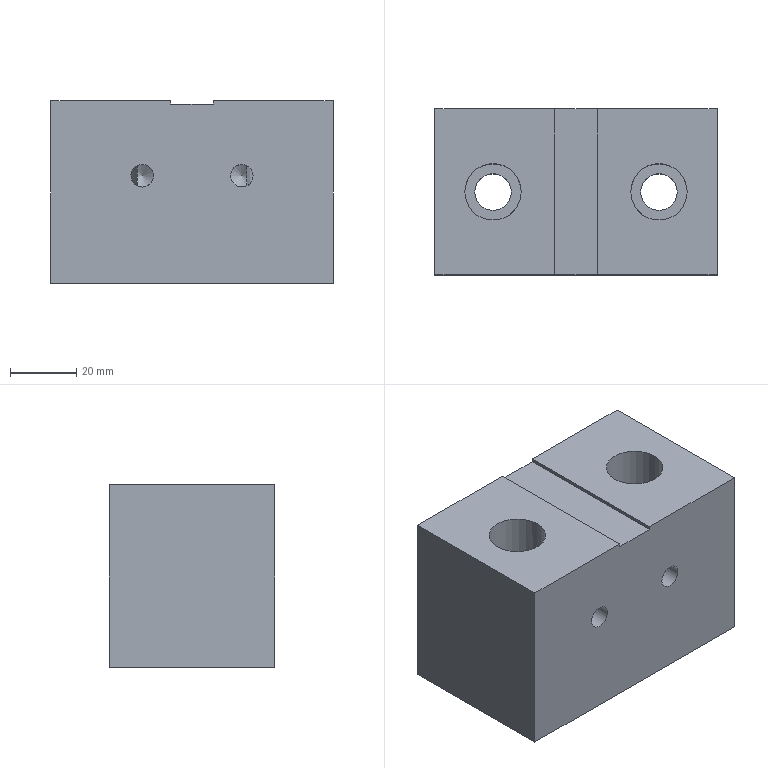Part | STEP file | 1 solid | 20 faces | box 85 x 50 x 55 mm | volume 210302 mm3 | plane 12 | cylinder 6 | cone 2 | commonest cylinder face diameters 6.8 x2 11 x2 17 x2
STEP:
#1=CARTESIAN_POINT('',(-370.,-292.5,-47.));
#2=VERTEX_POINT('',#1);
#3=CARTESIAN_POINT('',(-285.,-292.5,-47.));
#4=VERTEX_POINT('',#3);
#5=CARTESIAN_POINT('',(-383.,-292.5,-47.));
#6=DIRECTION('',(1.,0.,0.));
#7=VECTOR('',#6,1.);
#8=LINE('',#5,#7);
#9=EDGE_CURVE('',#2,#4,#8,.T.);
#10=ORIENTED_EDGE('',*,*,#9,.T.);
#11=CARTESIAN_POINT('',(-285.,-292.5,8.));
#12=VERTEX_POINT('',#11);
#13=CARTESIAN_POINT('',(-285.,-292.5,24.2));
#14=DIRECTION('',(0.,0.,1.));
#15=VECTOR('',#14,1.);
#16=LINE('',#13,#15);
#17=EDGE_CURVE('',#4,#12,#16,.T.);
#18=ORIENTED_EDGE('',*,*,#17,.T.);
#19=CARTESIAN_POINT('',(-321.15,-292.5,8.));
#20=VERTEX_POINT('',#19);
#21=CARTESIAN_POINT('',(-335.,-292.5,8.));
#22=DIRECTION('',(-1.,0.,0.));
#23=VECTOR('',#22,1.);
#24=LINE('',#21,#23);
#25=EDGE_CURVE('',#12,#20,#24,.T.);
#26=ORIENTED_EDGE('',*,*,#25,.T.);
#27=CARTESIAN_POINT('',(-321.15,-292.5,7.));
#28=VERTEX_POINT('',#27);
#29=CARTESIAN_POINT('',(-321.15,-292.5,24.2));
#30=DIRECTION('',(0.,0.,1.));
#31=VECTOR('',#30,1.);
#32=LINE('',#29,#31);
#33=EDGE_CURVE('',#28,#20,#32,.T.);
#34=ORIENTED_EDGE('',*,*,#33,.F.);
#35=CARTESIAN_POINT('',(-333.85,-292.5,7.));
#36=VERTEX_POINT('',#35);
#37=CARTESIAN_POINT('',(-383.,-292.5,7.));
#38=DIRECTION('',(1.,0.,0.));
#39=VECTOR('',#38,1.);
#40=LINE('',#37,#39);
#41=EDGE_CURVE('',#36,#28,#40,.T.);
#42=ORIENTED_EDGE('',*,*,#41,.F.);
#43=CARTESIAN_POINT('',(-333.85,-292.5,8.));
#44=VERTEX_POINT('',#43);
#45=CARTESIAN_POINT('',(-333.85,-292.5,24.2));
#46=DIRECTION('',(0.,0.,1.));
#47=VECTOR('',#46,1.);
#48=LINE('',#45,#47);
#49=EDGE_CURVE('',#36,#44,#48,.T.);
#50=ORIENTED_EDGE('',*,*,#49,.T.);
#51=CARTESIAN_POINT('',(-370.,-292.5,8.));
#52=VERTEX_POINT('',#51);
#53=CARTESIAN_POINT('',(-335.,-292.5,8.));
#54=DIRECTION('',(-1.,0.,0.));
#55=VECTOR('',#54,1.);
#56=LINE('',#53,#55);
#57=EDGE_CURVE('',#44,#52,#56,.T.);
#58=ORIENTED_EDGE('',*,*,#57,.T.);
#59=CARTESIAN_POINT('',(-370.,-292.5,24.2));
#60=DIRECTION('',(0.,0.,1.));
#61=VECTOR('',#60,1.);
#62=LINE('',#59,#61);
#63=EDGE_CURVE('',#2,#52,#62,.T.);
#64=ORIENTED_EDGE('',*,*,#63,.F.);
#65=EDGE_LOOP('',(#10,#18,#26,#34,#42,#50,#58,#64));
#66=FACE_BOUND('',#65,.T.);
#67=CARTESIAN_POINT('',(-339.1,-292.5,-14.6));
#68=VERTEX_POINT('',#67);
#69=CARTESIAN_POINT('',(-342.5,-292.5,-14.6));
#70=DIRECTION('',(0.,1.,0.));
#71=DIRECTION('',(1.,0.,0.));
#72=AXIS2_PLACEMENT_3D('',#69,#70,#71);
#73=CIRCLE('',#72,3.4);
#74=EDGE_CURVE('',#68,#68,#73,.T.);
#75=ORIENTED_EDGE('',*,*,#74,.T.);
#76=EDGE_LOOP('',(#75));
#77=FACE_BOUND('',#76,.T.);
#78=CARTESIAN_POINT('',(-309.1,-292.5,-14.6));
#79=VERTEX_POINT('',#78);
#80=CARTESIAN_POINT('',(-312.5,-292.5,-14.6));
#81=DIRECTION('',(0.,1.,0.));
#82=DIRECTION('',(1.,0.,0.));
#83=AXIS2_PLACEMENT_3D('',#80,#81,#82);
#84=CIRCLE('',#83,3.4);
#85=EDGE_CURVE('',#79,#79,#84,.T.);
#86=ORIENTED_EDGE('',*,*,#85,.T.);
#87=EDGE_LOOP('',(#86));
#88=FACE_BOUND('',#87,.T.);
#89=CARTESIAN_POINT('',(-383.,-292.5,24.2));
#90=DIRECTION('',(0.,-1.,0.));
#91=DIRECTION('',(0.,0.,-1.));
#92=AXIS2_PLACEMENT_3D('',#89,#90,#91);
#93=PLANE('',#92);
#94=ADVANCED_FACE('',(#66,#77,#88),#93,.T.);
#95=CARTESIAN_POINT('',(-361.,-267.5,8.));
#96=VERTEX_POINT('',#95);
#97=CARTESIAN_POINT('',(-352.5,-267.5,8.));
#98=DIRECTION('',(0.,0.,-1.));
#99=DIRECTION('',(-1.,0.,0.));
#100=AXIS2_PLACEMENT_3D('',#97,#98,#99);
#101=CIRCLE('',#100,8.5);
#102=EDGE_CURVE('',#96,#96,#101,.T.);
#103=ORIENTED_EDGE('',*,*,#102,.T.);
#104=EDGE_LOOP('',(#103));
#105=FACE_BOUND('',#104,.T.);
#106=CARTESIAN_POINT('',(-370.,-242.5,8.));
#107=VERTEX_POINT('',#106);
#108=CARTESIAN_POINT('',(-333.85,-242.5,8.));
#109=VERTEX_POINT('',#108);
#110=CARTESIAN_POINT('',(-335.,-242.5,8.));
#111=DIRECTION('',(1.,0.,0.));
#112=VECTOR('',#111,1.);
#113=LINE('',#110,#112);
#114=EDGE_CURVE('',#107,#109,#113,.T.);
#115=ORIENTED_EDGE('',*,*,#114,.F.);
#116=CARTESIAN_POINT('',(-370.,-513.,8.));
#117=DIRECTION('',(0.,1.,0.));
#118=VECTOR('',#117,1.);
#119=LINE('',#116,#118);
#120=EDGE_CURVE('',#52,#107,#119,.T.);
#121=ORIENTED_EDGE('',*,*,#120,.F.);
#122=ORIENTED_EDGE('',*,*,#57,.F.);
#123=CARTESIAN_POINT('',(-333.85,-513.,8.));
#124=DIRECTION('',(0.,-1.,0.));
#125=VECTOR('',#124,1.);
#126=LINE('',#123,#125);
#127=EDGE_CURVE('',#109,#44,#126,.T.);
#128=ORIENTED_EDGE('',*,*,#127,.F.);
#129=EDGE_LOOP('',(#115,#121,#122,#128));
#130=FACE_BOUND('',#129,.T.);
#131=CARTESIAN_POINT('',(-335.,-513.,8.));
#132=DIRECTION('',(0.,0.,-1.));
#133=DIRECTION('',(0.,1.,0.));
#134=AXIS2_PLACEMENT_3D('',#131,#132,#133);
#135=PLANE('',#134);
#136=ADVANCED_FACE('',(#105,#130),#135,.F.);
#137=ORIENTED_EDGE('',*,*,#120,.T.);
#138=CARTESIAN_POINT('',(-370.,-242.5,-47.));
#139=VERTEX_POINT('',#138);
#140=CARTESIAN_POINT('',(-370.,-242.5,24.2));
#141=DIRECTION('',(0.,0.,1.));
#142=VECTOR('',#141,1.);
#143=LINE('',#140,#142);
#144=EDGE_CURVE('',#139,#107,#143,.T.);
#145=ORIENTED_EDGE('',*,*,#144,.F.);
#146=CARTESIAN_POINT('',(-370.,-245.,-47.));
#147=DIRECTION('',(0.,-1.,0.));
#148=VECTOR('',#147,1.);
#149=LINE('',#146,#148);
#150=EDGE_CURVE('',#139,#2,#149,.T.);
#151=ORIENTED_EDGE('',*,*,#150,.T.);
#152=ORIENTED_EDGE('',*,*,#63,.T.);
#153=EDGE_LOOP('',(#137,#145,#151,#152));
#154=FACE_OUTER_BOUND('',#153,.T.);
#155=CARTESIAN_POINT('',(-370.,-245.,24.2));
#156=DIRECTION('',(-1.,0.,0.));
#157=DIRECTION('',(0.,0.,1.));
#158=AXIS2_PLACEMENT_3D('',#155,#156,#157);
#159=PLANE('',#158);
#160=ADVANCED_FACE('',(#154),#159,.T.);
#161=CARTESIAN_POINT('',(-321.15,-242.5,8.));
#162=VERTEX_POINT('',#161);
#163=CARTESIAN_POINT('',(-285.,-242.5,8.));
#164=VERTEX_POINT('',#163);
#165=CARTESIAN_POINT('',(-335.,-242.5,8.));
#166=DIRECTION('',(1.,0.,0.));
#167=VECTOR('',#166,1.);
#168=LINE('',#165,#167);
#169=EDGE_CURVE('',#162,#164,#168,.T.);
#170=ORIENTED_EDGE('',*,*,#169,.T.);
#171=CARTESIAN_POINT('',(-285.,-242.5,-47.));
#172=VERTEX_POINT('',#171);
#173=CARTESIAN_POINT('',(-285.,-242.5,24.2));
#174=DIRECTION('',(0.,0.,1.));
#175=VECTOR('',#174,1.);
#176=LINE('',#173,#175);
#177=EDGE_CURVE('',#172,#164,#176,.T.);
#178=ORIENTED_EDGE('',*,*,#177,.F.);
#179=CARTESIAN_POINT('',(-297.,-242.5,-47.));
#180=DIRECTION('',(-1.,0.,0.));
#181=VECTOR('',#180,1.);
#182=LINE('',#179,#181);
#183=EDGE_CURVE('',#172,#139,#182,.T.);
#184=ORIENTED_EDGE('',*,*,#183,.T.);
#185=ORIENTED_EDGE('',*,*,#144,.T.);
#186=ORIENTED_EDGE('',*,*,#114,.T.);
#187=CARTESIAN_POINT('',(-333.85,-242.5,7.));
#188=VERTEX_POINT('',#187);
#189=CARTESIAN_POINT('',(-333.85,-242.5,7.));
#190=DIRECTION('',(0.,0.,1.));
#191=VECTOR('',#190,1.);
#192=LINE('',#189,#191);
#193=EDGE_CURVE('',#188,#109,#192,.T.);
#194=ORIENTED_EDGE('',*,*,#193,.F.);
#195=CARTESIAN_POINT('',(-321.15,-242.5,7.));
#196=VERTEX_POINT('',#195);
#197=CARTESIAN_POINT('',(-327.5,-242.5,7.));
#198=DIRECTION('',(1.,0.,0.));
#199=VECTOR('',#198,1.);
#200=LINE('',#197,#199);
#201=EDGE_CURVE('',#188,#196,#200,.T.);
#202=ORIENTED_EDGE('',*,*,#201,.T.);
#203=CARTESIAN_POINT('',(-321.15,-242.5,7.));
#204=DIRECTION('',(0.,0.,1.));
#205=VECTOR('',#204,1.);
#206=LINE('',#203,#205);
#207=EDGE_CURVE('',#196,#162,#206,.T.);
#208=ORIENTED_EDGE('',*,*,#207,.T.);
#209=EDGE_LOOP('',(#170,#178,#184,#185,#186,#194,#202,#208));
#210=FACE_OUTER_BOUND('',#209,.T.);
#211=CARTESIAN_POINT('',(-297.,-242.5,24.2));
#212=DIRECTION('',(0.,1.,0.));
#213=DIRECTION('',(0.,0.,1.));
#214=AXIS2_PLACEMENT_3D('',#211,#212,#213);
#215=PLANE('',#214);
#216=ADVANCED_FACE('',(#210),#215,.T.);
#217=CARTESIAN_POINT('',(-285.,-291.,-47.));
#218=DIRECTION('',(0.,1.,0.));
#219=VECTOR('',#218,1.);
#220=LINE('',#217,#219);
#221=EDGE_CURVE('',#4,#172,#220,.T.);
#222=ORIENTED_EDGE('',*,*,#221,.T.);
#223=ORIENTED_EDGE('',*,*,#177,.T.);
#224=CARTESIAN_POINT('',(-285.,-513.,8.));
#225=DIRECTION('',(0.,-1.,0.));
#226=VECTOR('',#225,1.);
#227=LINE('',#224,#226);
#228=EDGE_CURVE('',#164,#12,#227,.T.);
#229=ORIENTED_EDGE('',*,*,#228,.T.);
#230=ORIENTED_EDGE('',*,*,#17,.F.);
#231=EDGE_LOOP('',(#222,#223,#229,#230));
#232=FACE_OUTER_BOUND('',#231,.T.);
#233=CARTESIAN_POINT('',(-285.,-291.,24.2));
#234=DIRECTION('',(1.,0.,0.));
#235=DIRECTION('',(0.,0.,-1.));
#236=AXIS2_PLACEMENT_3D('',#233,#234,#235);
#237=PLANE('',#236);
#238=ADVANCED_FACE('',(#232),#237,.T.);
#239=CARTESIAN_POINT('',(-311.,-267.5,8.));
#240=VERTEX_POINT('',#239);
#241=CARTESIAN_POINT('',(-302.5,-267.5,8.));
#242=DIRECTION('',(0.,0.,-1.));
#243=DIRECTION('',(-1.,0.,0.));
#244=AXIS2_PLACEMENT_3D('',#241,#242,#243);
#245=CIRCLE('',#244,8.5);
#246=EDGE_CURVE('',#240,#240,#245,.T.);
#247=ORIENTED_EDGE('',*,*,#246,.T.);
#248=EDGE_LOOP('',(#247));
#249=FACE_BOUND('',#248,.T.);
#250=ORIENTED_EDGE('',*,*,#228,.F.);
#251=ORIENTED_EDGE('',*,*,#169,.F.);
#252=CARTESIAN_POINT('',(-321.15,-513.,8.));
#253=DIRECTION('',(0.,-1.,0.));
#254=VECTOR('',#253,1.);
#255=LINE('',#252,#254);
#256=EDGE_CURVE('',#162,#20,#255,.T.);
#257=ORIENTED_EDGE('',*,*,#256,.T.);
#258=ORIENTED_EDGE('',*,*,#25,.F.);
#259=EDGE_LOOP('',(#250,#251,#257,#258));
#260=FACE_BOUND('',#259,.T.);
#261=CARTESIAN_POINT('',(-335.,-513.,8.));
#262=DIRECTION('',(0.,0.,-1.));
#263=DIRECTION('',(0.,1.,0.));
#264=AXIS2_PLACEMENT_3D('',#261,#262,#263);
#265=PLANE('',#264);
#266=ADVANCED_FACE('',(#249,#260),#265,.F.);
#267=CARTESIAN_POINT('',(-297.,-267.5,-47.));
#268=VERTEX_POINT('',#267);
#269=CARTESIAN_POINT('',(-302.5,-267.5,-47.));
#270=DIRECTION('',(0.,0.,1.));
#271=DIRECTION('',(1.,0.,0.));
#272=AXIS2_PLACEMENT_3D('',#269,#270,#271);
#273=CIRCLE('',#272,5.5);
#274=EDGE_CURVE('',#268,#268,#273,.T.);
#275=ORIENTED_EDGE('',*,*,#274,.T.);
#276=EDGE_LOOP('',(#275));
#277=FACE_BOUND('',#276,.T.);
#278=CARTESIAN_POINT('',(-347.,-267.5,-47.));
#279=VERTEX_POINT('',#278);
#280=CARTESIAN_POINT('',(-352.5,-267.5,-47.));
#281=DIRECTION('',(0.,0.,1.));
#282=DIRECTION('',(1.,0.,0.));
#283=AXIS2_PLACEMENT_3D('',#280,#281,#282);
#284=CIRCLE('',#283,5.5);
#285=EDGE_CURVE('',#279,#279,#284,.T.);
#286=ORIENTED_EDGE('',*,*,#285,.T.);
#287=EDGE_LOOP('',(#286));
#288=FACE_BOUND('',#287,.T.);
#289=ORIENTED_EDGE('',*,*,#183,.F.);
#290=ORIENTED_EDGE('',*,*,#221,.F.);
#291=ORIENTED_EDGE('',*,*,#9,.F.);
#292=ORIENTED_EDGE('',*,*,#150,.F.);
#293=EDGE_LOOP('',(#289,#290,#291,#292));
#294=FACE_BOUND('',#293,.T.);
#295=CARTESIAN_POINT('',(-335.,-513.,-47.));
#296=DIRECTION('',(0.,0.,-1.));
#297=DIRECTION('',(0.,1.,0.));
#298=AXIS2_PLACEMENT_3D('',#295,#296,#297);
#299=PLANE('',#298);
#300=ADVANCED_FACE('',(#277,#288,#294),#299,.T.);
#301=ORIENTED_EDGE('',*,*,#207,.F.);
#302=CARTESIAN_POINT('',(-321.15,-297.5,7.));
#303=DIRECTION('',(0.,-1.,0.));
#304=VECTOR('',#303,1.);
#305=LINE('',#302,#304);
#306=EDGE_CURVE('',#196,#28,#305,.T.);
#307=ORIENTED_EDGE('',*,*,#306,.T.);
#308=ORIENTED_EDGE('',*,*,#33,.T.);
#309=ORIENTED_EDGE('',*,*,#256,.F.);
#310=EDGE_LOOP('',(#301,#307,#308,#309));
#311=FACE_OUTER_BOUND('',#310,.T.);
#312=CARTESIAN_POINT('',(-321.15,-297.5,7.));
#313=DIRECTION('',(1.,0.,0.));
#314=DIRECTION('',(0.,1.,0.));
#315=AXIS2_PLACEMENT_3D('',#312,#313,#314);
#316=PLANE('',#315);
#317=ADVANCED_FACE('',(#311),#316,.F.);
#318=ORIENTED_EDGE('',*,*,#127,.T.);
#319=ORIENTED_EDGE('',*,*,#49,.F.);
#320=CARTESIAN_POINT('',(-333.85,-297.5,7.));
#321=DIRECTION('',(0.,-1.,0.));
#322=VECTOR('',#321,1.);
#323=LINE('',#320,#322);
#324=EDGE_CURVE('',#188,#36,#323,.T.);
#325=ORIENTED_EDGE('',*,*,#324,.F.);
#326=ORIENTED_EDGE('',*,*,#193,.T.);
#327=EDGE_LOOP('',(#318,#319,#325,#326));
#328=FACE_OUTER_BOUND('',#327,.T.);
#329=CARTESIAN_POINT('',(-333.85,-297.5,7.));
#330=DIRECTION('',(1.,0.,0.));
#331=DIRECTION('',(0.,1.,0.));
#332=AXIS2_PLACEMENT_3D('',#329,#330,#331);
#333=PLANE('',#332);
#334=ADVANCED_FACE('',(#328),#333,.T.);
#335=ORIENTED_EDGE('',*,*,#41,.T.);
#336=ORIENTED_EDGE('',*,*,#306,.F.);
#337=ORIENTED_EDGE('',*,*,#201,.F.);
#338=ORIENTED_EDGE('',*,*,#324,.T.);
#339=EDGE_LOOP('',(#335,#336,#337,#338));
#340=FACE_OUTER_BOUND('',#339,.T.);
#341=CARTESIAN_POINT('',(-327.5,-297.5,7.));
#342=DIRECTION('',(0.,0.,-1.));
#343=DIRECTION('',(0.,1.,0.));
#344=AXIS2_PLACEMENT_3D('',#341,#342,#343);
#345=PLANE('',#344);
#346=ADVANCED_FACE('',(#340),#345,.F.);
#347=CARTESIAN_POINT('',(-358.,-267.5,-32.));
#348=VERTEX_POINT('',#347);
#349=CARTESIAN_POINT('',(-352.5,-267.5,-32.));
#350=DIRECTION('',(0.,0.,-1.));
#351=DIRECTION('',(-1.,0.,0.));
#352=AXIS2_PLACEMENT_3D('',#349,#350,#351);
#353=CIRCLE('',#352,5.5);
#354=EDGE_CURVE('',#348,#348,#353,.T.);
#355=ORIENTED_EDGE('',*,*,#354,.F.);
#356=EDGE_LOOP('',(#355));
#357=FACE_BOUND('',#356,.T.);
#358=ORIENTED_EDGE('',*,*,#285,.F.);
#359=EDGE_LOOP('',(#358));
#360=FACE_BOUND('',#359,.T.);
#361=CARTESIAN_POINT('',(-352.5,-267.5,-47.));
#362=DIRECTION('',(0.,0.,1.));
#363=DIRECTION('',(1.,0.,0.));
#364=AXIS2_PLACEMENT_3D('',#361,#362,#363);
#365=CYLINDRICAL_SURFACE('',#364,5.5);
#366=ADVANCED_FACE('',(#357,#360),#365,.F.);
#367=ORIENTED_EDGE('',*,*,#354,.T.);
#368=EDGE_LOOP('',(#367));
#369=FACE_BOUND('',#368,.T.);
#370=CARTESIAN_POINT('',(-344.,-267.5,-32.));
#371=VERTEX_POINT('',#370);
#372=CARTESIAN_POINT('',(-352.5,-267.5,-32.));
#373=DIRECTION('',(0.,0.,-1.));
#374=DIRECTION('',(1.,0.,0.));
#375=AXIS2_PLACEMENT_3D('',#372,#373,#374);
#376=CIRCLE('',#375,8.5);
#377=EDGE_CURVE('',#371,#371,#376,.T.);
#378=ORIENTED_EDGE('',*,*,#377,.F.);
#379=EDGE_LOOP('',(#378));
#380=FACE_BOUND('',#379,.T.);
#381=CARTESIAN_POINT('',(-352.5,-267.5,-32.));
#382=DIRECTION('',(0.,0.,-1.));
#383=DIRECTION('',(-1.,0.,0.));
#384=AXIS2_PLACEMENT_3D('',#381,#382,#383);
#385=PLANE('',#384);
#386=ADVANCED_FACE('',(#369,#380),#385,.F.);
#387=CARTESIAN_POINT('',(-344.,-267.5,-17.651));
#388=VERTEX_POINT('',#387);
#389=CARTESIAN_POINT('',(-344.,-267.5,-11.549));
#390=VERTEX_POINT('',#389);
#391=CARTESIAN_POINT('',(-344.,-267.5,-17.651));
#392=CARTESIAN_POINT('',(-344.,-266.99,-16.685));
#393=CARTESIAN_POINT('',(-344.069,-266.419,-15.675));
#394=CARTESIAN_POINT('',(-344.068,-266.426,-13.505));
#395=CARTESIAN_POINT('',(-344.,-266.993,-12.51));
#396=CARTESIAN_POINT('',(-344.,-267.5,-11.549));
#397=B_SPLINE_CURVE_WITH_KNOTS('',3,(#391,#392,#393,#394,#395,#396),.UNSPECIFIED.,.F.,.F.,(4,2,4),(0.,0.5,1.),.UNSPECIFIED.);
#398=EDGE_CURVE('',#388,#390,#397,.T.);
#399=ORIENTED_EDGE('',*,*,#398,.T.);
#400=CARTESIAN_POINT('',(-344.,-267.5,-11.549));
#401=CARTESIAN_POINT('',(-344.,-268.712,-11.549));
#402=CARTESIAN_POINT('',(-344.272,-269.917,-11.635));
#403=CARTESIAN_POINT('',(-344.964,-271.473,-12.238));
#404=CARTESIAN_POINT('',(-345.245,-271.949,-12.534));
#405=CARTESIAN_POINT('',(-345.721,-272.645,-13.403));
#406=CARTESIAN_POINT('',(-345.899,-272.855,-13.992));
#407=CARTESIAN_POINT('',(-345.901,-272.857,-15.2));
#408=CARTESIAN_POINT('',(-345.723,-272.647,-15.792));
#409=CARTESIAN_POINT('',(-345.246,-271.951,-16.666));
#410=CARTESIAN_POINT('',(-344.966,-271.475,-16.961));
#411=CARTESIAN_POINT('',(-344.273,-269.921,-17.565));
#412=CARTESIAN_POINT('',(-344.,-268.713,-17.651));
#413=CARTESIAN_POINT('',(-344.,-267.5,-17.651));
#414=B_SPLINE_CURVE_WITH_KNOTS('',3,(#400,#401,#402,#403,#404,#405,#406,#407,#408,#409,#410,#411,#412,#413),.UNSPECIFIED.,.F.,.F.,(4,2,2,2,2,2,4),(0.,0.25,0.375,0.5,0.625,0.75,1.),.UNSPECIFIED.);
#415=EDGE_CURVE('',#390,#388,#414,.T.);
#416=ORIENTED_EDGE('',*,*,#415,.T.);
#417=EDGE_LOOP('',(#399,#416));
#418=FACE_BOUND('',#417,.T.);
#419=ORIENTED_EDGE('',*,*,#102,.F.);
#420=EDGE_LOOP('',(#419));
#421=FACE_BOUND('',#420,.T.);
#422=ORIENTED_EDGE('',*,*,#377,.T.);
#423=EDGE_LOOP('',(#422));
#424=FACE_BOUND('',#423,.T.);
#425=CARTESIAN_POINT('',(-352.5,-267.5,-32.));
#426=DIRECTION('',(0.,0.,1.));
#427=DIRECTION('',(1.,0.,0.));
#428=AXIS2_PLACEMENT_3D('',#425,#426,#427);
#429=CYLINDRICAL_SURFACE('',#428,8.5);
#430=ADVANCED_FACE('',(#418,#421,#424),#429,.F.);
#431=CARTESIAN_POINT('',(-308.,-267.5,-32.));
#432=VERTEX_POINT('',#431);
#433=CARTESIAN_POINT('',(-302.5,-267.5,-32.));
#434=DIRECTION('',(0.,0.,-1.));
#435=DIRECTION('',(-1.,0.,0.));
#436=AXIS2_PLACEMENT_3D('',#433,#434,#435);
#437=CIRCLE('',#436,5.5);
#438=EDGE_CURVE('',#432,#432,#437,.T.);
#439=ORIENTED_EDGE('',*,*,#438,.F.);
#440=EDGE_LOOP('',(#439));
#441=FACE_BOUND('',#440,.T.);
#442=ORIENTED_EDGE('',*,*,#274,.F.);
#443=EDGE_LOOP('',(#442));
#444=FACE_BOUND('',#443,.T.);
#445=CARTESIAN_POINT('',(-302.5,-267.5,-47.));
#446=DIRECTION('',(0.,0.,1.));
#447=DIRECTION('',(1.,0.,0.));
#448=AXIS2_PLACEMENT_3D('',#445,#446,#447);
#449=CYLINDRICAL_SURFACE('',#448,5.5);
#450=ADVANCED_FACE('',(#441,#444),#449,.F.);
#451=ORIENTED_EDGE('',*,*,#438,.T.);
#452=EDGE_LOOP('',(#451));
#453=FACE_BOUND('',#452,.T.);
#454=CARTESIAN_POINT('',(-294.,-267.5,-32.));
#455=VERTEX_POINT('',#454);
#456=CARTESIAN_POINT('',(-302.5,-267.5,-32.));
#457=DIRECTION('',(0.,0.,-1.));
#458=DIRECTION('',(1.,0.,0.));
#459=AXIS2_PLACEMENT_3D('',#456,#457,#458);
#460=CIRCLE('',#459,8.5);
#461=EDGE_CURVE('',#455,#455,#460,.T.);
#462=ORIENTED_EDGE('',*,*,#461,.F.);
#463=EDGE_LOOP('',(#462));
#464=FACE_BOUND('',#463,.T.);
#465=CARTESIAN_POINT('',(-302.5,-267.5,-32.));
#466=DIRECTION('',(0.,0.,-1.));
#467=DIRECTION('',(-1.,0.,0.));
#468=AXIS2_PLACEMENT_3D('',#465,#466,#467);
#469=PLANE('',#468);
#470=ADVANCED_FACE('',(#453,#464),#469,.F.);
#471=CARTESIAN_POINT('',(-311.,-267.5,-11.549));
#472=VERTEX_POINT('',#471);
#473=CARTESIAN_POINT('',(-311.,-267.5,-17.651));
#474=VERTEX_POINT('',#473);
#475=CARTESIAN_POINT('',(-311.,-267.5,-11.549));
#476=CARTESIAN_POINT('',(-311.,-266.99,-12.515));
#477=CARTESIAN_POINT('',(-310.931,-266.419,-13.525));
#478=CARTESIAN_POINT('',(-310.932,-266.426,-15.695));
#479=CARTESIAN_POINT('',(-311.,-266.993,-16.69));
#480=CARTESIAN_POINT('',(-311.,-267.5,-17.651));
#481=B_SPLINE_CURVE_WITH_KNOTS('',3,(#475,#476,#477,#478,#479,#480),.UNSPECIFIED.,.F.,.F.,(4,2,4),(0.,0.5,1.),.UNSPECIFIED.);
#482=EDGE_CURVE('',#472,#474,#481,.T.);
#483=ORIENTED_EDGE('',*,*,#482,.T.);
#484=CARTESIAN_POINT('',(-311.,-267.5,-17.651));
#485=CARTESIAN_POINT('',(-311.,-268.712,-17.651));
#486=CARTESIAN_POINT('',(-310.728,-269.917,-17.565));
#487=CARTESIAN_POINT('',(-310.036,-271.473,-16.962));
#488=CARTESIAN_POINT('',(-309.755,-271.949,-16.666));
#489=CARTESIAN_POINT('',(-309.279,-272.645,-15.797));
#490=CARTESIAN_POINT('',(-309.101,-272.855,-15.208));
#491=CARTESIAN_POINT('',(-309.099,-272.857,-14.));
#492=CARTESIAN_POINT('',(-309.277,-272.647,-13.408));
#493=CARTESIAN_POINT('',(-309.754,-271.951,-12.534));
#494=CARTESIAN_POINT('',(-310.034,-271.475,-12.239));
#495=CARTESIAN_POINT('',(-310.727,-269.921,-11.635));
#496=CARTESIAN_POINT('',(-311.,-268.713,-11.549));
#497=CARTESIAN_POINT('',(-311.,-267.5,-11.549));
#498=B_SPLINE_CURVE_WITH_KNOTS('',3,(#484,#485,#486,#487,#488,#489,#490,#491,#492,#493,#494,#495,#496,#497),.UNSPECIFIED.,.F.,.F.,(4,2,2,2,2,2,4),(0.,0.25,0.375,0.5,0.625,0.75,1.),.UNSPECIFIED.);
#499=EDGE_CURVE('',#474,#472,#498,.T.);
#500=ORIENTED_EDGE('',*,*,#499,.T.);
#501=EDGE_LOOP('',(#483,#500));
#502=FACE_BOUND('',#501,.T.);
#503=ORIENTED_EDGE('',*,*,#246,.F.);
#504=EDGE_LOOP('',(#503));
#505=FACE_BOUND('',#504,.T.);
#506=ORIENTED_EDGE('',*,*,#461,.T.);
#507=EDGE_LOOP('',(#506));
#508=FACE_BOUND('',#507,.T.);
#509=CARTESIAN_POINT('',(-302.5,-267.5,-32.));
#510=DIRECTION('',(0.,0.,1.));
#511=DIRECTION('',(1.,0.,0.));
#512=AXIS2_PLACEMENT_3D('',#509,#510,#511);
#513=CYLINDRICAL_SURFACE('',#512,8.5);
#514=ADVANCED_FACE('',(#502,#505,#508),#513,.F.);
#515=ORIENTED_EDGE('',*,*,#74,.F.);
#516=EDGE_LOOP('',(#515));
#517=FACE_BOUND('',#516,.T.);
#518=CARTESIAN_POINT('',(-342.5,-267.5,-14.6));
#519=DIRECTION('',(0.,-1.,0.));
#520=DIRECTION('',(-1.,0.,0.));
#521=AXIS2_PLACEMENT_3D('',#518,#519,#520);
#522=CIRCLE('',#521,3.4);
#523=EDGE_CURVE('',#388,#390,#522,.T.);
#524=ORIENTED_EDGE('',*,*,#523,.F.);
#525=ORIENTED_EDGE('',*,*,#415,.F.);
#526=EDGE_LOOP('',(#524,#525));
#527=FACE_BOUND('',#526,.T.);
#528=CARTESIAN_POINT('',(-342.5,-292.5,-14.6));
#529=DIRECTION('',(0.,1.,0.));
#530=DIRECTION('',(-1.,0.,0.));
#531=AXIS2_PLACEMENT_3D('',#528,#529,#530);
#532=CYLINDRICAL_SURFACE('',#531,3.4);
#533=ADVANCED_FACE('',(#517,#527),#532,.F.);
#534=CARTESIAN_POINT('',(-342.5,-265.5,-14.6));
#535=VERTEX_POINT('',#534);
#536=VERTEX_LOOP('',#535);
#537=FACE_BOUND('',#536,.T.);
#538=ORIENTED_EDGE('',*,*,#523,.T.);
#539=ORIENTED_EDGE('',*,*,#398,.F.);
#540=EDGE_LOOP('',(#538,#539));
#541=FACE_BOUND('',#540,.T.);
#542=CARTESIAN_POINT('',(-342.5,-265.5,-14.6));
#543=DIRECTION('',(0.,-1.,0.));
#544=DIRECTION('',(-1.,0.,0.));
#545=AXIS2_PLACEMENT_3D('',#542,#543,#544);
#546=CONICAL_SURFACE('',#545,0.,59.534);
#547=ADVANCED_FACE('',(#537,#541),#546,.F.);
#548=ORIENTED_EDGE('',*,*,#85,.F.);
#549=EDGE_LOOP('',(#548));
#550=FACE_BOUND('',#549,.T.);
#551=CARTESIAN_POINT('',(-312.5,-267.5,-14.6));
#552=DIRECTION('',(0.,-1.,0.));
#553=DIRECTION('',(-1.,0.,0.));
#554=AXIS2_PLACEMENT_3D('',#551,#552,#553);
#555=CIRCLE('',#554,3.4);
#556=EDGE_CURVE('',#472,#474,#555,.T.);
#557=ORIENTED_EDGE('',*,*,#556,.F.);
#558=ORIENTED_EDGE('',*,*,#499,.F.);
#559=EDGE_LOOP('',(#557,#558));
#560=FACE_BOUND('',#559,.T.);
#561=CARTESIAN_POINT('',(-312.5,-292.5,-14.6));
#562=DIRECTION('',(0.,1.,0.));
#563=DIRECTION('',(-1.,0.,0.));
#564=AXIS2_PLACEMENT_3D('',#561,#562,#563);
#565=CYLINDRICAL_SURFACE('',#564,3.4);
#566=ADVANCED_FACE('',(#550,#560),#565,.F.);
#567=CARTESIAN_POINT('',(-312.5,-265.5,-14.6));
#568=VERTEX_POINT('',#567);
#569=VERTEX_LOOP('',#568);
#570=FACE_BOUND('',#569,.T.);
#571=ORIENTED_EDGE('',*,*,#556,.T.);
#572=ORIENTED_EDGE('',*,*,#482,.F.);
#573=EDGE_LOOP('',(#571,#572));
#574=FACE_BOUND('',#573,.T.);
#575=CARTESIAN_POINT('',(-312.5,-265.5,-14.6));
#576=DIRECTION('',(0.,-1.,0.));
#577=DIRECTION('',(-1.,0.,0.));
#578=AXIS2_PLACEMENT_3D('',#575,#576,#577);
#579=CONICAL_SURFACE('',#578,0.,59.534);
#580=ADVANCED_FACE('',(#570,#574),#579,.F.);
#581=CLOSED_SHELL('',(#94,#136,#160,#216,#238,#266,#300,#317,#334,#346,#366,#386,#430,#450,#470,#514,#533,#547,#566,#580));
#582=MANIFOLD_SOLID_BREP('',#581);
#583=(LENGTH_UNIT()NAMED_UNIT(*)SI_UNIT(.MILLI.,.METRE.));
#584=UNCERTAINTY_MEASURE_WITH_UNIT(LENGTH_MEASURE(0.0508),#583,'','');
#585=(NAMED_UNIT(*)PLANE_ANGLE_UNIT()SI_UNIT($,.RADIAN.));
#586=PLANE_ANGLE_MEASURE_WITH_UNIT(PLANE_ANGLE_MEASURE(0.01745),#585);
#587=DIMENSIONAL_EXPONENTS(0.,0.,0.,0.,0.,0.,0.);
#588=(CONVERSION_BASED_UNIT('DEGREE',#586)NAMED_UNIT(#587)PLANE_ANGLE_UNIT());
#589=(NAMED_UNIT(*)SI_UNIT($,.STERADIAN.)SOLID_ANGLE_UNIT());
#590=(GEOMETRIC_REPRESENTATION_CONTEXT(3)GLOBAL_UNCERTAINTY_ASSIGNED_CONTEXT((#584))GLOBAL_UNIT_ASSIGNED_CONTEXT((#583,#588,#589))REPRESENTATION_CONTEXT('',''));
#591=ADVANCED_BREP_SHAPE_REPRESENTATION('',(#582),#590);